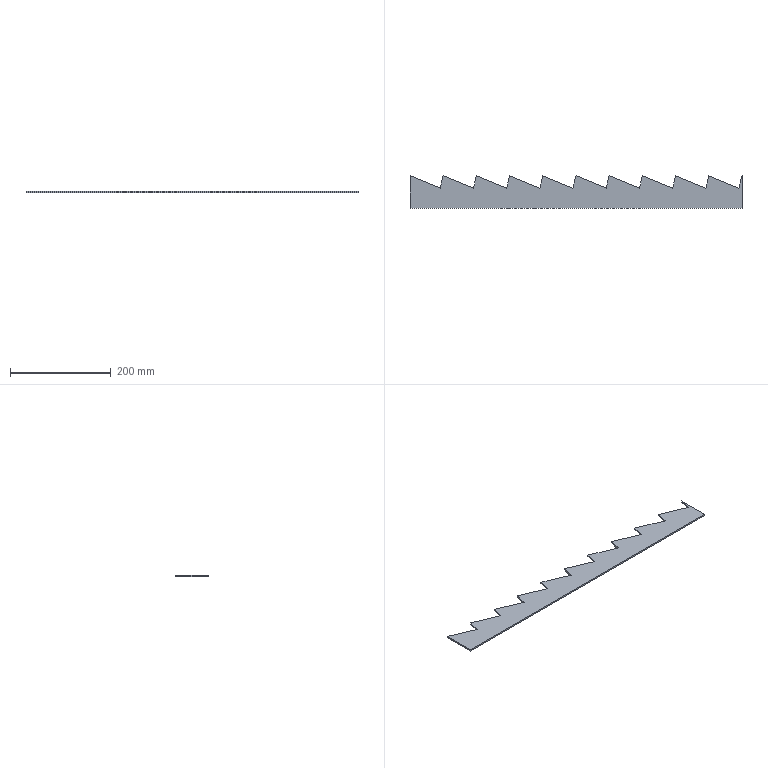Part | SolidWorks | features BaseBody 1 | 1 solid | 25 faces | box 660 x 65 x 3 mm | volume 103950 mm3 | plane 25
STEP:
#1=CARTESIAN_POINT('',(660.,-65.,0.));
#2=VERTEX_POINT('',#1);
#3=CARTESIAN_POINT('',(660.,0.,0.));
#4=VERTEX_POINT('',#3);
#5=CARTESIAN_POINT('',(660.,-32.5,0.));
#6=DIRECTION('',(0.,1.,0.));
#7=VECTOR('',#6,1000.);
#8=LINE('',#5,#7);
#9=EDGE_CURVE('',#2,#4,#8,.T.);
#10=ORIENTED_EDGE('',*,*,#9,.F.);
#11=CARTESIAN_POINT('',(0.,-65.,0.));
#12=VERTEX_POINT('',#11);
#13=CARTESIAN_POINT('',(330.,-65.,0.));
#14=DIRECTION('',(1.,0.,0.));
#15=VECTOR('',#14,1000.);
#16=LINE('',#13,#15);
#17=EDGE_CURVE('',#12,#2,#16,.T.);
#18=ORIENTED_EDGE('',*,*,#17,.F.);
#19=CARTESIAN_POINT('',(0.,0.,0.));
#20=VERTEX_POINT('',#19);
#21=CARTESIAN_POINT('',(0.,-32.5,0.));
#22=DIRECTION('',(0.,-1.,0.));
#23=VECTOR('',#22,1000.);
#24=LINE('',#21,#23);
#25=EDGE_CURVE('',#20,#12,#24,.T.);
#26=ORIENTED_EDGE('',*,*,#25,.F.);
#27=CARTESIAN_POINT('',(60.,-25.,0.));
#28=VERTEX_POINT('',#27);
#29=CARTESIAN_POINT('',(60.,-25.,0.));
#30=DIRECTION('',(-0.9231,0.3846,0.));
#31=VECTOR('',#30,1000.);
#32=LINE('',#29,#31);
#33=EDGE_CURVE('',#28,#20,#32,.T.);
#34=ORIENTED_EDGE('',*,*,#33,.F.);
#35=CARTESIAN_POINT('',(66.,0.,0.));
#36=VERTEX_POINT('',#35);
#37=CARTESIAN_POINT('',(66.,0.,0.));
#38=DIRECTION('',(-0.2334,-0.9724,0.));
#39=VECTOR('',#38,1000.);
#40=LINE('',#37,#39);
#41=EDGE_CURVE('',#36,#28,#40,.T.);
#42=ORIENTED_EDGE('',*,*,#41,.F.);
#43=CARTESIAN_POINT('',(126.,-25.,0.));
#44=VERTEX_POINT('',#43);
#45=CARTESIAN_POINT('',(126.,-25.,0.));
#46=DIRECTION('',(-0.9231,0.3846,0.));
#47=VECTOR('',#46,1000.);
#48=LINE('',#45,#47);
#49=EDGE_CURVE('',#44,#36,#48,.T.);
#50=ORIENTED_EDGE('',*,*,#49,.F.);
#51=CARTESIAN_POINT('',(132.,0.,0.));
#52=VERTEX_POINT('',#51);
#53=CARTESIAN_POINT('',(132.,0.,0.));
#54=DIRECTION('',(-0.2334,-0.9724,0.));
#55=VECTOR('',#54,1000.);
#56=LINE('',#53,#55);
#57=EDGE_CURVE('',#52,#44,#56,.T.);
#58=ORIENTED_EDGE('',*,*,#57,.F.);
#59=CARTESIAN_POINT('',(192.,-25.,0.));
#60=VERTEX_POINT('',#59);
#61=CARTESIAN_POINT('',(192.,-25.,0.));
#62=DIRECTION('',(-0.9231,0.3846,0.));
#63=VECTOR('',#62,1000.);
#64=LINE('',#61,#63);
#65=EDGE_CURVE('',#60,#52,#64,.T.);
#66=ORIENTED_EDGE('',*,*,#65,.F.);
#67=CARTESIAN_POINT('',(198.,0.,0.));
#68=VERTEX_POINT('',#67);
#69=CARTESIAN_POINT('',(198.,0.,0.));
#70=DIRECTION('',(-0.2334,-0.9724,0.));
#71=VECTOR('',#70,1000.);
#72=LINE('',#69,#71);
#73=EDGE_CURVE('',#68,#60,#72,.T.);
#74=ORIENTED_EDGE('',*,*,#73,.F.);
#75=CARTESIAN_POINT('',(258.,-25.,0.));
#76=VERTEX_POINT('',#75);
#77=CARTESIAN_POINT('',(258.,-25.,0.));
#78=DIRECTION('',(-0.9231,0.3846,0.));
#79=VECTOR('',#78,1000.);
#80=LINE('',#77,#79);
#81=EDGE_CURVE('',#76,#68,#80,.T.);
#82=ORIENTED_EDGE('',*,*,#81,.F.);
#83=CARTESIAN_POINT('',(264.,0.,0.));
#84=VERTEX_POINT('',#83);
#85=CARTESIAN_POINT('',(264.,0.,0.));
#86=DIRECTION('',(-0.2334,-0.9724,0.));
#87=VECTOR('',#86,1000.);
#88=LINE('',#85,#87);
#89=EDGE_CURVE('',#84,#76,#88,.T.);
#90=ORIENTED_EDGE('',*,*,#89,.F.);
#91=CARTESIAN_POINT('',(324.,-25.,0.));
#92=VERTEX_POINT('',#91);
#93=CARTESIAN_POINT('',(324.,-25.,0.));
#94=DIRECTION('',(-0.9231,0.3846,0.));
#95=VECTOR('',#94,1000.);
#96=LINE('',#93,#95);
#97=EDGE_CURVE('',#92,#84,#96,.T.);
#98=ORIENTED_EDGE('',*,*,#97,.F.);
#99=CARTESIAN_POINT('',(330.,0.,0.));
#100=VERTEX_POINT('',#99);
#101=CARTESIAN_POINT('',(330.,0.,0.));
#102=DIRECTION('',(-0.2334,-0.9724,0.));
#103=VECTOR('',#102,1000.);
#104=LINE('',#101,#103);
#105=EDGE_CURVE('',#100,#92,#104,.T.);
#106=ORIENTED_EDGE('',*,*,#105,.F.);
#107=CARTESIAN_POINT('',(390.,-25.,0.));
#108=VERTEX_POINT('',#107);
#109=CARTESIAN_POINT('',(390.,-25.,0.));
#110=DIRECTION('',(-0.9231,0.3846,0.));
#111=VECTOR('',#110,1000.);
#112=LINE('',#109,#111);
#113=EDGE_CURVE('',#108,#100,#112,.T.);
#114=ORIENTED_EDGE('',*,*,#113,.F.);
#115=CARTESIAN_POINT('',(396.,0.,0.));
#116=VERTEX_POINT('',#115);
#117=CARTESIAN_POINT('',(396.,0.,0.));
#118=DIRECTION('',(-0.2334,-0.9724,0.));
#119=VECTOR('',#118,1000.);
#120=LINE('',#117,#119);
#121=EDGE_CURVE('',#116,#108,#120,.T.);
#122=ORIENTED_EDGE('',*,*,#121,.F.);
#123=CARTESIAN_POINT('',(456.,-25.,0.));
#124=VERTEX_POINT('',#123);
#125=CARTESIAN_POINT('',(456.,-25.,0.));
#126=DIRECTION('',(-0.9231,0.3846,0.));
#127=VECTOR('',#126,1000.);
#128=LINE('',#125,#127);
#129=EDGE_CURVE('',#124,#116,#128,.T.);
#130=ORIENTED_EDGE('',*,*,#129,.F.);
#131=CARTESIAN_POINT('',(462.,0.,0.));
#132=VERTEX_POINT('',#131);
#133=CARTESIAN_POINT('',(462.,0.,0.));
#134=DIRECTION('',(-0.2334,-0.9724,0.));
#135=VECTOR('',#134,1000.);
#136=LINE('',#133,#135);
#137=EDGE_CURVE('',#132,#124,#136,.T.);
#138=ORIENTED_EDGE('',*,*,#137,.F.);
#139=CARTESIAN_POINT('',(522.,-25.,0.));
#140=VERTEX_POINT('',#139);
#141=CARTESIAN_POINT('',(522.,-25.,0.));
#142=DIRECTION('',(-0.9231,0.3846,0.));
#143=VECTOR('',#142,1000.);
#144=LINE('',#141,#143);
#145=EDGE_CURVE('',#140,#132,#144,.T.);
#146=ORIENTED_EDGE('',*,*,#145,.F.);
#147=CARTESIAN_POINT('',(528.,0.,0.));
#148=VERTEX_POINT('',#147);
#149=CARTESIAN_POINT('',(528.,0.,0.));
#150=DIRECTION('',(-0.2334,-0.9724,0.));
#151=VECTOR('',#150,1000.);
#152=LINE('',#149,#151);
#153=EDGE_CURVE('',#148,#140,#152,.T.);
#154=ORIENTED_EDGE('',*,*,#153,.F.);
#155=CARTESIAN_POINT('',(588.,-25.,0.));
#156=VERTEX_POINT('',#155);
#157=CARTESIAN_POINT('',(588.,-25.,0.));
#158=DIRECTION('',(-0.9231,0.3846,0.));
#159=VECTOR('',#158,1000.);
#160=LINE('',#157,#159);
#161=EDGE_CURVE('',#156,#148,#160,.T.);
#162=ORIENTED_EDGE('',*,*,#161,.F.);
#163=CARTESIAN_POINT('',(594.,0.,0.));
#164=VERTEX_POINT('',#163);
#165=CARTESIAN_POINT('',(594.,0.,0.));
#166=DIRECTION('',(-0.2334,-0.9724,0.));
#167=VECTOR('',#166,1000.);
#168=LINE('',#165,#167);
#169=EDGE_CURVE('',#164,#156,#168,.T.);
#170=ORIENTED_EDGE('',*,*,#169,.F.);
#171=CARTESIAN_POINT('',(654.,-25.,0.));
#172=VERTEX_POINT('',#171);
#173=CARTESIAN_POINT('',(654.,-25.,0.));
#174=DIRECTION('',(-0.9231,0.3846,0.));
#175=VECTOR('',#174,1000.);
#176=LINE('',#173,#175);
#177=EDGE_CURVE('',#172,#164,#176,.T.);
#178=ORIENTED_EDGE('',*,*,#177,.F.);
#179=CARTESIAN_POINT('',(660.,0.,0.));
#180=DIRECTION('',(-0.2334,-0.9724,0.));
#181=VECTOR('',#180,1000.);
#182=LINE('',#179,#181);
#183=EDGE_CURVE('',#4,#172,#182,.T.);
#184=ORIENTED_EDGE('',*,*,#183,.F.);
#185=EDGE_LOOP('',(#10,#18,#26,#34,#42,#50,#58,#66,#74,#82,#90,#98,#106,#114,#122,#130,#138,#146,#154,#162,#170,#178,#184));
#186=FACE_OUTER_BOUND('',#185,.T.);
#187=CARTESIAN_POINT('',(330.,-32.5,0.));
#188=DIRECTION('',(0.,0.,1.));
#189=DIRECTION('',(1.,0.,0.));
#190=AXIS2_PLACEMENT_3D('',#187,#188,#189);
#191=PLANE('',#190);
#192=ADVANCED_FACE('',(#186),#191,.F.);
#193=CARTESIAN_POINT('',(654.,-25.,3.));
#194=VERTEX_POINT('',#193);
#195=CARTESIAN_POINT('',(654.,-25.,3.));
#196=DIRECTION('',(0.,0.,-1.));
#197=VECTOR('',#196,1000.);
#198=LINE('',#195,#197);
#199=EDGE_CURVE('',#194,#172,#198,.T.);
#200=ORIENTED_EDGE('',*,*,#199,.F.);
#201=CARTESIAN_POINT('',(660.,0.,3.));
#202=VERTEX_POINT('',#201);
#203=CARTESIAN_POINT('',(660.,0.,3.));
#204=DIRECTION('',(-0.2334,-0.9724,0.));
#205=VECTOR('',#204,1000.);
#206=LINE('',#203,#205);
#207=EDGE_CURVE('',#202,#194,#206,.T.);
#208=ORIENTED_EDGE('',*,*,#207,.F.);
#209=CARTESIAN_POINT('',(660.,0.,3.));
#210=DIRECTION('',(0.,0.,1.));
#211=VECTOR('',#210,1000.);
#212=LINE('',#209,#211);
#213=EDGE_CURVE('',#4,#202,#212,.T.);
#214=ORIENTED_EDGE('',*,*,#213,.F.);
#215=ORIENTED_EDGE('',*,*,#183,.T.);
#216=EDGE_LOOP('',(#200,#208,#214,#215));
#217=FACE_OUTER_BOUND('',#216,.T.);
#218=CARTESIAN_POINT('',(660.,0.,3.));
#219=DIRECTION('',(0.9724,-0.2334,0.));
#220=DIRECTION('',(0.2334,0.9724,0.));
#221=AXIS2_PLACEMENT_3D('',#218,#219,#220);
#222=PLANE('',#221);
#223=ADVANCED_FACE('',(#217),#222,.F.);
#224=CARTESIAN_POINT('',(660.,-65.,3.));
#225=VERTEX_POINT('',#224);
#226=CARTESIAN_POINT('',(660.,-65.,3.));
#227=DIRECTION('',(0.,-1.,0.));
#228=VECTOR('',#227,1000.);
#229=LINE('',#226,#228);
#230=EDGE_CURVE('',#202,#225,#229,.T.);
#231=ORIENTED_EDGE('',*,*,#230,.T.);
#232=CARTESIAN_POINT('',(660.,-65.,0.));
#233=DIRECTION('',(0.,0.,-1.));
#234=VECTOR('',#233,1000.);
#235=LINE('',#232,#234);
#236=EDGE_CURVE('',#225,#2,#235,.T.);
#237=ORIENTED_EDGE('',*,*,#236,.T.);
#238=ORIENTED_EDGE('',*,*,#9,.T.);
#239=ORIENTED_EDGE('',*,*,#213,.T.);
#240=EDGE_LOOP('',(#231,#237,#238,#239));
#241=FACE_OUTER_BOUND('',#240,.T.);
#242=CARTESIAN_POINT('',(660.,-65.,0.));
#243=DIRECTION('',(1.,0.,0.));
#244=DIRECTION('',(0.,0.,-1.));
#245=AXIS2_PLACEMENT_3D('',#242,#243,#244);
#246=PLANE('',#245);
#247=ADVANCED_FACE('',(#241),#246,.T.);
#248=CARTESIAN_POINT('',(0.,-65.,3.));
#249=VERTEX_POINT('',#248);
#250=CARTESIAN_POINT('',(0.,-65.,3.));
#251=DIRECTION('',(-1.,0.,0.));
#252=VECTOR('',#251,1000.);
#253=LINE('',#250,#252);
#254=EDGE_CURVE('',#225,#249,#253,.T.);
#255=ORIENTED_EDGE('',*,*,#254,.T.);
#256=CARTESIAN_POINT('',(0.,-65.,0.));
#257=DIRECTION('',(0.,0.,-1.));
#258=VECTOR('',#257,1000.);
#259=LINE('',#256,#258);
#260=EDGE_CURVE('',#249,#12,#259,.T.);
#261=ORIENTED_EDGE('',*,*,#260,.T.);
#262=ORIENTED_EDGE('',*,*,#17,.T.);
#263=ORIENTED_EDGE('',*,*,#236,.F.);
#264=EDGE_LOOP('',(#255,#261,#262,#263));
#265=FACE_OUTER_BOUND('',#264,.T.);
#266=CARTESIAN_POINT('',(0.,-65.,0.));
#267=DIRECTION('',(0.,-1.,0.));
#268=DIRECTION('',(1.,0.,0.));
#269=AXIS2_PLACEMENT_3D('',#266,#267,#268);
#270=PLANE('',#269);
#271=ADVANCED_FACE('',(#265),#270,.T.);
#272=CARTESIAN_POINT('',(0.,0.,3.));
#273=VERTEX_POINT('',#272);
#274=CARTESIAN_POINT('',(0.,0.,3.));
#275=DIRECTION('',(0.,1.,0.));
#276=VECTOR('',#275,1000.);
#277=LINE('',#274,#276);
#278=EDGE_CURVE('',#249,#273,#277,.T.);
#279=ORIENTED_EDGE('',*,*,#278,.T.);
#280=CARTESIAN_POINT('',(0.,0.,0.));
#281=DIRECTION('',(0.,0.,-1.));
#282=VECTOR('',#281,1000.);
#283=LINE('',#280,#282);
#284=EDGE_CURVE('',#273,#20,#283,.T.);
#285=ORIENTED_EDGE('',*,*,#284,.T.);
#286=ORIENTED_EDGE('',*,*,#25,.T.);
#287=ORIENTED_EDGE('',*,*,#260,.F.);
#288=EDGE_LOOP('',(#279,#285,#286,#287));
#289=FACE_OUTER_BOUND('',#288,.T.);
#290=CARTESIAN_POINT('',(0.,0.,0.));
#291=DIRECTION('',(-1.,0.,0.));
#292=DIRECTION('',(0.,-1.,0.));
#293=AXIS2_PLACEMENT_3D('',#290,#291,#292);
#294=PLANE('',#293);
#295=ADVANCED_FACE('',(#289),#294,.T.);
#296=ORIENTED_EDGE('',*,*,#284,.F.);
#297=CARTESIAN_POINT('',(60.,-25.,3.));
#298=VERTEX_POINT('',#297);
#299=CARTESIAN_POINT('',(60.,-25.,3.));
#300=DIRECTION('',(-0.9231,0.3846,0.));
#301=VECTOR('',#300,1000.);
#302=LINE('',#299,#301);
#303=EDGE_CURVE('',#298,#273,#302,.T.);
#304=ORIENTED_EDGE('',*,*,#303,.F.);
#305=CARTESIAN_POINT('',(60.,-25.,3.));
#306=DIRECTION('',(0.,0.,1.));
#307=VECTOR('',#306,1000.);
#308=LINE('',#305,#307);
#309=EDGE_CURVE('',#28,#298,#308,.T.);
#310=ORIENTED_EDGE('',*,*,#309,.F.);
#311=ORIENTED_EDGE('',*,*,#33,.T.);
#312=EDGE_LOOP('',(#296,#304,#310,#311));
#313=FACE_OUTER_BOUND('',#312,.T.);
#314=CARTESIAN_POINT('',(60.,-25.,3.));
#315=DIRECTION('',(-0.3846,-0.9231,0.));
#316=DIRECTION('',(0.9231,-0.3846,0.));
#317=AXIS2_PLACEMENT_3D('',#314,#315,#316);
#318=PLANE('',#317);
#319=ADVANCED_FACE('',(#313),#318,.F.);
#320=ORIENTED_EDGE('',*,*,#309,.T.);
#321=CARTESIAN_POINT('',(66.,0.,3.));
#322=VERTEX_POINT('',#321);
#323=CARTESIAN_POINT('',(66.,0.,3.));
#324=DIRECTION('',(-0.2334,-0.9724,0.));
#325=VECTOR('',#324,1000.);
#326=LINE('',#323,#325);
#327=EDGE_CURVE('',#322,#298,#326,.T.);
#328=ORIENTED_EDGE('',*,*,#327,.F.);
#329=CARTESIAN_POINT('',(66.,0.,3.));
#330=DIRECTION('',(0.,0.,1.));
#331=VECTOR('',#330,1000.);
#332=LINE('',#329,#331);
#333=EDGE_CURVE('',#36,#322,#332,.T.);
#334=ORIENTED_EDGE('',*,*,#333,.F.);
#335=ORIENTED_EDGE('',*,*,#41,.T.);
#336=EDGE_LOOP('',(#320,#328,#334,#335));
#337=FACE_OUTER_BOUND('',#336,.T.);
#338=CARTESIAN_POINT('',(66.,0.,3.));
#339=DIRECTION('',(0.9724,-0.2334,0.));
#340=DIRECTION('',(0.2334,0.9724,0.));
#341=AXIS2_PLACEMENT_3D('',#338,#339,#340);
#342=PLANE('',#341);
#343=ADVANCED_FACE('',(#337),#342,.F.);
#344=ORIENTED_EDGE('',*,*,#333,.T.);
#345=CARTESIAN_POINT('',(126.,-25.,3.));
#346=VERTEX_POINT('',#345);
#347=CARTESIAN_POINT('',(126.,-25.,3.));
#348=DIRECTION('',(-0.9231,0.3846,0.));
#349=VECTOR('',#348,1000.);
#350=LINE('',#347,#349);
#351=EDGE_CURVE('',#346,#322,#350,.T.);
#352=ORIENTED_EDGE('',*,*,#351,.F.);
#353=CARTESIAN_POINT('',(126.,-25.,3.));
#354=DIRECTION('',(0.,0.,1.));
#355=VECTOR('',#354,1000.);
#356=LINE('',#353,#355);
#357=EDGE_CURVE('',#44,#346,#356,.T.);
#358=ORIENTED_EDGE('',*,*,#357,.F.);
#359=ORIENTED_EDGE('',*,*,#49,.T.);
#360=EDGE_LOOP('',(#344,#352,#358,#359));
#361=FACE_OUTER_BOUND('',#360,.T.);
#362=CARTESIAN_POINT('',(126.,-25.,3.));
#363=DIRECTION('',(-0.3846,-0.9231,0.));
#364=DIRECTION('',(0.9231,-0.3846,0.));
#365=AXIS2_PLACEMENT_3D('',#362,#363,#364);
#366=PLANE('',#365);
#367=ADVANCED_FACE('',(#361),#366,.F.);
#368=ORIENTED_EDGE('',*,*,#357,.T.);
#369=CARTESIAN_POINT('',(132.,0.,3.));
#370=VERTEX_POINT('',#369);
#371=CARTESIAN_POINT('',(132.,0.,3.));
#372=DIRECTION('',(-0.2334,-0.9724,0.));
#373=VECTOR('',#372,1000.);
#374=LINE('',#371,#373);
#375=EDGE_CURVE('',#370,#346,#374,.T.);
#376=ORIENTED_EDGE('',*,*,#375,.F.);
#377=CARTESIAN_POINT('',(132.,0.,3.));
#378=DIRECTION('',(0.,0.,1.));
#379=VECTOR('',#378,1000.);
#380=LINE('',#377,#379);
#381=EDGE_CURVE('',#52,#370,#380,.T.);
#382=ORIENTED_EDGE('',*,*,#381,.F.);
#383=ORIENTED_EDGE('',*,*,#57,.T.);
#384=EDGE_LOOP('',(#368,#376,#382,#383));
#385=FACE_OUTER_BOUND('',#384,.T.);
#386=CARTESIAN_POINT('',(132.,0.,3.));
#387=DIRECTION('',(0.9724,-0.2334,0.));
#388=DIRECTION('',(0.2334,0.9724,0.));
#389=AXIS2_PLACEMENT_3D('',#386,#387,#388);
#390=PLANE('',#389);
#391=ADVANCED_FACE('',(#385),#390,.F.);
#392=ORIENTED_EDGE('',*,*,#381,.T.);
#393=CARTESIAN_POINT('',(192.,-25.,3.));
#394=VERTEX_POINT('',#393);
#395=CARTESIAN_POINT('',(192.,-25.,3.));
#396=DIRECTION('',(-0.9231,0.3846,0.));
#397=VECTOR('',#396,1000.);
#398=LINE('',#395,#397);
#399=EDGE_CURVE('',#394,#370,#398,.T.);
#400=ORIENTED_EDGE('',*,*,#399,.F.);
#401=CARTESIAN_POINT('',(192.,-25.,3.));
#402=DIRECTION('',(0.,0.,1.));
#403=VECTOR('',#402,1000.);
#404=LINE('',#401,#403);
#405=EDGE_CURVE('',#60,#394,#404,.T.);
#406=ORIENTED_EDGE('',*,*,#405,.F.);
#407=ORIENTED_EDGE('',*,*,#65,.T.);
#408=EDGE_LOOP('',(#392,#400,#406,#407));
#409=FACE_OUTER_BOUND('',#408,.T.);
#410=CARTESIAN_POINT('',(192.,-25.,3.));
#411=DIRECTION('',(-0.3846,-0.9231,0.));
#412=DIRECTION('',(0.9231,-0.3846,0.));
#413=AXIS2_PLACEMENT_3D('',#410,#411,#412);
#414=PLANE('',#413);
#415=ADVANCED_FACE('',(#409),#414,.F.);
#416=ORIENTED_EDGE('',*,*,#405,.T.);
#417=CARTESIAN_POINT('',(198.,0.,3.));
#418=VERTEX_POINT('',#417);
#419=CARTESIAN_POINT('',(198.,0.,3.));
#420=DIRECTION('',(-0.2334,-0.9724,0.));
#421=VECTOR('',#420,1000.);
#422=LINE('',#419,#421);
#423=EDGE_CURVE('',#418,#394,#422,.T.);
#424=ORIENTED_EDGE('',*,*,#423,.F.);
#425=CARTESIAN_POINT('',(198.,0.,3.));
#426=DIRECTION('',(0.,0.,1.));
#427=VECTOR('',#426,1000.);
#428=LINE('',#425,#427);
#429=EDGE_CURVE('',#68,#418,#428,.T.);
#430=ORIENTED_EDGE('',*,*,#429,.F.);
#431=ORIENTED_EDGE('',*,*,#73,.T.);
#432=EDGE_LOOP('',(#416,#424,#430,#431));
#433=FACE_OUTER_BOUND('',#432,.T.);
#434=CARTESIAN_POINT('',(198.,0.,3.));
#435=DIRECTION('',(0.9724,-0.2334,0.));
#436=DIRECTION('',(0.2334,0.9724,0.));
#437=AXIS2_PLACEMENT_3D('',#434,#435,#436);
#438=PLANE('',#437);
#439=ADVANCED_FACE('',(#433),#438,.F.);
#440=ORIENTED_EDGE('',*,*,#429,.T.);
#441=CARTESIAN_POINT('',(258.,-25.,3.));
#442=VERTEX_POINT('',#441);
#443=CARTESIAN_POINT('',(258.,-25.,3.));
#444=DIRECTION('',(-0.9231,0.3846,0.));
#445=VECTOR('',#444,1000.);
#446=LINE('',#443,#445);
#447=EDGE_CURVE('',#442,#418,#446,.T.);
#448=ORIENTED_EDGE('',*,*,#447,.F.);
#449=CARTESIAN_POINT('',(258.,-25.,3.));
#450=DIRECTION('',(0.,0.,1.));
#451=VECTOR('',#450,1000.);
#452=LINE('',#449,#451);
#453=EDGE_CURVE('',#76,#442,#452,.T.);
#454=ORIENTED_EDGE('',*,*,#453,.F.);
#455=ORIENTED_EDGE('',*,*,#81,.T.);
#456=EDGE_LOOP('',(#440,#448,#454,#455));
#457=FACE_OUTER_BOUND('',#456,.T.);
#458=CARTESIAN_POINT('',(258.,-25.,3.));
#459=DIRECTION('',(-0.3846,-0.9231,0.));
#460=DIRECTION('',(0.9231,-0.3846,0.));
#461=AXIS2_PLACEMENT_3D('',#458,#459,#460);
#462=PLANE('',#461);
#463=ADVANCED_FACE('',(#457),#462,.F.);
#464=ORIENTED_EDGE('',*,*,#453,.T.);
#465=CARTESIAN_POINT('',(264.,0.,3.));
#466=VERTEX_POINT('',#465);
#467=CARTESIAN_POINT('',(264.,0.,3.));
#468=DIRECTION('',(-0.2334,-0.9724,0.));
#469=VECTOR('',#468,1000.);
#470=LINE('',#467,#469);
#471=EDGE_CURVE('',#466,#442,#470,.T.);
#472=ORIENTED_EDGE('',*,*,#471,.F.);
#473=CARTESIAN_POINT('',(264.,0.,3.));
#474=DIRECTION('',(0.,0.,1.));
#475=VECTOR('',#474,1000.);
#476=LINE('',#473,#475);
#477=EDGE_CURVE('',#84,#466,#476,.T.);
#478=ORIENTED_EDGE('',*,*,#477,.F.);
#479=ORIENTED_EDGE('',*,*,#89,.T.);
#480=EDGE_LOOP('',(#464,#472,#478,#479));
#481=FACE_OUTER_BOUND('',#480,.T.);
#482=CARTESIAN_POINT('',(264.,0.,3.));
#483=DIRECTION('',(0.9724,-0.2334,0.));
#484=DIRECTION('',(0.2334,0.9724,0.));
#485=AXIS2_PLACEMENT_3D('',#482,#483,#484);
#486=PLANE('',#485);
#487=ADVANCED_FACE('',(#481),#486,.F.);
#488=ORIENTED_EDGE('',*,*,#477,.T.);
#489=CARTESIAN_POINT('',(324.,-25.,3.));
#490=VERTEX_POINT('',#489);
#491=CARTESIAN_POINT('',(324.,-25.,3.));
#492=DIRECTION('',(-0.9231,0.3846,0.));
#493=VECTOR('',#492,1000.);
#494=LINE('',#491,#493);
#495=EDGE_CURVE('',#490,#466,#494,.T.);
#496=ORIENTED_EDGE('',*,*,#495,.F.);
#497=CARTESIAN_POINT('',(324.,-25.,3.));
#498=DIRECTION('',(0.,0.,1.));
#499=VECTOR('',#498,1000.);
#500=LINE('',#497,#499);
#501=EDGE_CURVE('',#92,#490,#500,.T.);
#502=ORIENTED_EDGE('',*,*,#501,.F.);
#503=ORIENTED_EDGE('',*,*,#97,.T.);
#504=EDGE_LOOP('',(#488,#496,#502,#503));
#505=FACE_OUTER_BOUND('',#504,.T.);
#506=CARTESIAN_POINT('',(324.,-25.,3.));
#507=DIRECTION('',(-0.3846,-0.9231,0.));
#508=DIRECTION('',(0.9231,-0.3846,0.));
#509=AXIS2_PLACEMENT_3D('',#506,#507,#508);
#510=PLANE('',#509);
#511=ADVANCED_FACE('',(#505),#510,.F.);
#512=ORIENTED_EDGE('',*,*,#501,.T.);
#513=CARTESIAN_POINT('',(330.,0.,3.));
#514=VERTEX_POINT('',#513);
#515=CARTESIAN_POINT('',(330.,0.,3.));
#516=DIRECTION('',(-0.2334,-0.9724,0.));
#517=VECTOR('',#516,1000.);
#518=LINE('',#515,#517);
#519=EDGE_CURVE('',#514,#490,#518,.T.);
#520=ORIENTED_EDGE('',*,*,#519,.F.);
#521=CARTESIAN_POINT('',(330.,0.,3.));
#522=DIRECTION('',(0.,0.,1.));
#523=VECTOR('',#522,1000.);
#524=LINE('',#521,#523);
#525=EDGE_CURVE('',#100,#514,#524,.T.);
#526=ORIENTED_EDGE('',*,*,#525,.F.);
#527=ORIENTED_EDGE('',*,*,#105,.T.);
#528=EDGE_LOOP('',(#512,#520,#526,#527));
#529=FACE_OUTER_BOUND('',#528,.T.);
#530=CARTESIAN_POINT('',(330.,0.,3.));
#531=DIRECTION('',(0.9724,-0.2334,0.));
#532=DIRECTION('',(0.2334,0.9724,0.));
#533=AXIS2_PLACEMENT_3D('',#530,#531,#532);
#534=PLANE('',#533);
#535=ADVANCED_FACE('',(#529),#534,.F.);
#536=ORIENTED_EDGE('',*,*,#525,.T.);
#537=CARTESIAN_POINT('',(390.,-25.,3.));
#538=VERTEX_POINT('',#537);
#539=CARTESIAN_POINT('',(390.,-25.,3.));
#540=DIRECTION('',(-0.9231,0.3846,0.));
#541=VECTOR('',#540,1000.);
#542=LINE('',#539,#541);
#543=EDGE_CURVE('',#538,#514,#542,.T.);
#544=ORIENTED_EDGE('',*,*,#543,.F.);
#545=CARTESIAN_POINT('',(390.,-25.,3.));
#546=DIRECTION('',(0.,0.,1.));
#547=VECTOR('',#546,1000.);
#548=LINE('',#545,#547);
#549=EDGE_CURVE('',#108,#538,#548,.T.);
#550=ORIENTED_EDGE('',*,*,#549,.F.);
#551=ORIENTED_EDGE('',*,*,#113,.T.);
#552=EDGE_LOOP('',(#536,#544,#550,#551));
#553=FACE_OUTER_BOUND('',#552,.T.);
#554=CARTESIAN_POINT('',(390.,-25.,3.));
#555=DIRECTION('',(-0.3846,-0.9231,0.));
#556=DIRECTION('',(0.9231,-0.3846,0.));
#557=AXIS2_PLACEMENT_3D('',#554,#555,#556);
#558=PLANE('',#557);
#559=ADVANCED_FACE('',(#553),#558,.F.);
#560=ORIENTED_EDGE('',*,*,#549,.T.);
#561=CARTESIAN_POINT('',(396.,0.,3.));
#562=VERTEX_POINT('',#561);
#563=CARTESIAN_POINT('',(396.,0.,3.));
#564=DIRECTION('',(-0.2334,-0.9724,0.));
#565=VECTOR('',#564,1000.);
#566=LINE('',#563,#565);
#567=EDGE_CURVE('',#562,#538,#566,.T.);
#568=ORIENTED_EDGE('',*,*,#567,.F.);
#569=CARTESIAN_POINT('',(396.,0.,3.));
#570=DIRECTION('',(0.,0.,1.));
#571=VECTOR('',#570,1000.);
#572=LINE('',#569,#571);
#573=EDGE_CURVE('',#116,#562,#572,.T.);
#574=ORIENTED_EDGE('',*,*,#573,.F.);
#575=ORIENTED_EDGE('',*,*,#121,.T.);
#576=EDGE_LOOP('',(#560,#568,#574,#575));
#577=FACE_OUTER_BOUND('',#576,.T.);
#578=CARTESIAN_POINT('',(396.,0.,3.));
#579=DIRECTION('',(0.9724,-0.2334,0.));
#580=DIRECTION('',(0.2334,0.9724,0.));
#581=AXIS2_PLACEMENT_3D('',#578,#579,#580);
#582=PLANE('',#581);
#583=ADVANCED_FACE('',(#577),#582,.F.);
#584=ORIENTED_EDGE('',*,*,#573,.T.);
#585=CARTESIAN_POINT('',(456.,-25.,3.));
#586=VERTEX_POINT('',#585);
#587=CARTESIAN_POINT('',(456.,-25.,3.));
#588=DIRECTION('',(-0.9231,0.3846,0.));
#589=VECTOR('',#588,1000.);
#590=LINE('',#587,#589);
#591=EDGE_CURVE('',#586,#562,#590,.T.);
#592=ORIENTED_EDGE('',*,*,#591,.F.);
#593=CARTESIAN_POINT('',(456.,-25.,3.));
#594=DIRECTION('',(0.,0.,1.));
#595=VECTOR('',#594,1000.);
#596=LINE('',#593,#595);
#597=EDGE_CURVE('',#124,#586,#596,.T.);
#598=ORIENTED_EDGE('',*,*,#597,.F.);
#599=ORIENTED_EDGE('',*,*,#129,.T.);
#600=EDGE_LOOP('',(#584,#592,#598,#599));
#601=FACE_OUTER_BOUND('',#600,.T.);
#602=CARTESIAN_POINT('',(456.,-25.,3.));
#603=DIRECTION('',(-0.3846,-0.9231,0.));
#604=DIRECTION('',(0.9231,-0.3846,0.));
#605=AXIS2_PLACEMENT_3D('',#602,#603,#604);
#606=PLANE('',#605);
#607=ADVANCED_FACE('',(#601),#606,.F.);
#608=ORIENTED_EDGE('',*,*,#597,.T.);
#609=CARTESIAN_POINT('',(462.,0.,3.));
#610=VERTEX_POINT('',#609);
#611=CARTESIAN_POINT('',(462.,0.,3.));
#612=DIRECTION('',(-0.2334,-0.9724,0.));
#613=VECTOR('',#612,1000.);
#614=LINE('',#611,#613);
#615=EDGE_CURVE('',#610,#586,#614,.T.);
#616=ORIENTED_EDGE('',*,*,#615,.F.);
#617=CARTESIAN_POINT('',(462.,0.,3.));
#618=DIRECTION('',(0.,0.,1.));
#619=VECTOR('',#618,1000.);
#620=LINE('',#617,#619);
#621=EDGE_CURVE('',#132,#610,#620,.T.);
#622=ORIENTED_EDGE('',*,*,#621,.F.);
#623=ORIENTED_EDGE('',*,*,#137,.T.);
#624=EDGE_LOOP('',(#608,#616,#622,#623));
#625=FACE_OUTER_BOUND('',#624,.T.);
#626=CARTESIAN_POINT('',(462.,0.,3.));
#627=DIRECTION('',(0.9724,-0.2334,0.));
#628=DIRECTION('',(0.2334,0.9724,0.));
#629=AXIS2_PLACEMENT_3D('',#626,#627,#628);
#630=PLANE('',#629);
#631=ADVANCED_FACE('',(#625),#630,.F.);
#632=ORIENTED_EDGE('',*,*,#621,.T.);
#633=CARTESIAN_POINT('',(522.,-25.,3.));
#634=VERTEX_POINT('',#633);
#635=CARTESIAN_POINT('',(522.,-25.,3.));
#636=DIRECTION('',(-0.9231,0.3846,0.));
#637=VECTOR('',#636,1000.);
#638=LINE('',#635,#637);
#639=EDGE_CURVE('',#634,#610,#638,.T.);
#640=ORIENTED_EDGE('',*,*,#639,.F.);
#641=CARTESIAN_POINT('',(522.,-25.,3.));
#642=DIRECTION('',(0.,0.,1.));
#643=VECTOR('',#642,1000.);
#644=LINE('',#641,#643);
#645=EDGE_CURVE('',#140,#634,#644,.T.);
#646=ORIENTED_EDGE('',*,*,#645,.F.);
#647=ORIENTED_EDGE('',*,*,#145,.T.);
#648=EDGE_LOOP('',(#632,#640,#646,#647));
#649=FACE_OUTER_BOUND('',#648,.T.);
#650=CARTESIAN_POINT('',(522.,-25.,3.));
#651=DIRECTION('',(-0.3846,-0.9231,0.));
#652=DIRECTION('',(0.9231,-0.3846,0.));
#653=AXIS2_PLACEMENT_3D('',#650,#651,#652);
#654=PLANE('',#653);
#655=ADVANCED_FACE('',(#649),#654,.F.);
#656=ORIENTED_EDGE('',*,*,#645,.T.);
#657=CARTESIAN_POINT('',(528.,0.,3.));
#658=VERTEX_POINT('',#657);
#659=CARTESIAN_POINT('',(528.,0.,3.));
#660=DIRECTION('',(-0.2334,-0.9724,0.));
#661=VECTOR('',#660,1000.);
#662=LINE('',#659,#661);
#663=EDGE_CURVE('',#658,#634,#662,.T.);
#664=ORIENTED_EDGE('',*,*,#663,.F.);
#665=CARTESIAN_POINT('',(528.,0.,3.));
#666=DIRECTION('',(0.,0.,1.));
#667=VECTOR('',#666,1000.);
#668=LINE('',#665,#667);
#669=EDGE_CURVE('',#148,#658,#668,.T.);
#670=ORIENTED_EDGE('',*,*,#669,.F.);
#671=ORIENTED_EDGE('',*,*,#153,.T.);
#672=EDGE_LOOP('',(#656,#664,#670,#671));
#673=FACE_OUTER_BOUND('',#672,.T.);
#674=CARTESIAN_POINT('',(528.,0.,3.));
#675=DIRECTION('',(0.9724,-0.2334,0.));
#676=DIRECTION('',(0.2334,0.9724,0.));
#677=AXIS2_PLACEMENT_3D('',#674,#675,#676);
#678=PLANE('',#677);
#679=ADVANCED_FACE('',(#673),#678,.F.);
#680=ORIENTED_EDGE('',*,*,#669,.T.);
#681=CARTESIAN_POINT('',(588.,-25.,3.));
#682=VERTEX_POINT('',#681);
#683=CARTESIAN_POINT('',(588.,-25.,3.));
#684=DIRECTION('',(-0.9231,0.3846,0.));
#685=VECTOR('',#684,1000.);
#686=LINE('',#683,#685);
#687=EDGE_CURVE('',#682,#658,#686,.T.);
#688=ORIENTED_EDGE('',*,*,#687,.F.);
#689=CARTESIAN_POINT('',(588.,-25.,3.));
#690=DIRECTION('',(0.,0.,1.));
#691=VECTOR('',#690,1000.);
#692=LINE('',#689,#691);
#693=EDGE_CURVE('',#156,#682,#692,.T.);
#694=ORIENTED_EDGE('',*,*,#693,.F.);
#695=ORIENTED_EDGE('',*,*,#161,.T.);
#696=EDGE_LOOP('',(#680,#688,#694,#695));
#697=FACE_OUTER_BOUND('',#696,.T.);
#698=CARTESIAN_POINT('',(588.,-25.,3.));
#699=DIRECTION('',(-0.3846,-0.9231,0.));
#700=DIRECTION('',(0.9231,-0.3846,0.));
#701=AXIS2_PLACEMENT_3D('',#698,#699,#700);
#702=PLANE('',#701);
#703=ADVANCED_FACE('',(#697),#702,.F.);
#704=ORIENTED_EDGE('',*,*,#693,.T.);
#705=CARTESIAN_POINT('',(594.,0.,3.));
#706=VERTEX_POINT('',#705);
#707=CARTESIAN_POINT('',(594.,0.,3.));
#708=DIRECTION('',(-0.2334,-0.9724,0.));
#709=VECTOR('',#708,1000.);
#710=LINE('',#707,#709);
#711=EDGE_CURVE('',#706,#682,#710,.T.);
#712=ORIENTED_EDGE('',*,*,#711,.F.);
#713=CARTESIAN_POINT('',(594.,0.,3.));
#714=DIRECTION('',(0.,0.,1.));
#715=VECTOR('',#714,1000.);
#716=LINE('',#713,#715);
#717=EDGE_CURVE('',#164,#706,#716,.T.);
#718=ORIENTED_EDGE('',*,*,#717,.F.);
#719=ORIENTED_EDGE('',*,*,#169,.T.);
#720=EDGE_LOOP('',(#704,#712,#718,#719));
#721=FACE_OUTER_BOUND('',#720,.T.);
#722=CARTESIAN_POINT('',(594.,0.,3.));
#723=DIRECTION('',(0.9724,-0.2334,0.));
#724=DIRECTION('',(0.2334,0.9724,0.));
#725=AXIS2_PLACEMENT_3D('',#722,#723,#724);
#726=PLANE('',#725);
#727=ADVANCED_FACE('',(#721),#726,.F.);
#728=ORIENTED_EDGE('',*,*,#717,.T.);
#729=CARTESIAN_POINT('',(654.,-25.,3.));
#730=DIRECTION('',(-0.9231,0.3846,0.));
#731=VECTOR('',#730,1000.);
#732=LINE('',#729,#731);
#733=EDGE_CURVE('',#194,#706,#732,.T.);
#734=ORIENTED_EDGE('',*,*,#733,.F.);
#735=ORIENTED_EDGE('',*,*,#199,.T.);
#736=ORIENTED_EDGE('',*,*,#177,.T.);
#737=EDGE_LOOP('',(#728,#734,#735,#736));
#738=FACE_OUTER_BOUND('',#737,.T.);
#739=CARTESIAN_POINT('',(654.,-25.,3.));
#740=DIRECTION('',(-0.3846,-0.9231,0.));
#741=DIRECTION('',(0.9231,-0.3846,0.));
#742=AXIS2_PLACEMENT_3D('',#739,#740,#741);
#743=PLANE('',#742);
#744=ADVANCED_FACE('',(#738),#743,.F.);
#745=ORIENTED_EDGE('',*,*,#254,.F.);
#746=ORIENTED_EDGE('',*,*,#230,.F.);
#747=ORIENTED_EDGE('',*,*,#207,.T.);
#748=ORIENTED_EDGE('',*,*,#733,.T.);
#749=ORIENTED_EDGE('',*,*,#711,.T.);
#750=ORIENTED_EDGE('',*,*,#687,.T.);
#751=ORIENTED_EDGE('',*,*,#663,.T.);
#752=ORIENTED_EDGE('',*,*,#639,.T.);
#753=ORIENTED_EDGE('',*,*,#615,.T.);
#754=ORIENTED_EDGE('',*,*,#591,.T.);
#755=ORIENTED_EDGE('',*,*,#567,.T.);
#756=ORIENTED_EDGE('',*,*,#543,.T.);
#757=ORIENTED_EDGE('',*,*,#519,.T.);
#758=ORIENTED_EDGE('',*,*,#495,.T.);
#759=ORIENTED_EDGE('',*,*,#471,.T.);
#760=ORIENTED_EDGE('',*,*,#447,.T.);
#761=ORIENTED_EDGE('',*,*,#423,.T.);
#762=ORIENTED_EDGE('',*,*,#399,.T.);
#763=ORIENTED_EDGE('',*,*,#375,.T.);
#764=ORIENTED_EDGE('',*,*,#351,.T.);
#765=ORIENTED_EDGE('',*,*,#327,.T.);
#766=ORIENTED_EDGE('',*,*,#303,.T.);
#767=ORIENTED_EDGE('',*,*,#278,.F.);
#768=EDGE_LOOP('',(#745,#746,#747,#748,#749,#750,#751,#752,#753,#754,#755,#756,#757,#758,#759,#760,#761,#762,#763,#764,#765,#766,#767));
#769=FACE_OUTER_BOUND('',#768,.T.);
#770=CARTESIAN_POINT('',(330.,-32.5,3.));
#771=DIRECTION('',(0.,0.,1.));
#772=DIRECTION('',(1.,0.,0.));
#773=AXIS2_PLACEMENT_3D('',#770,#771,#772);
#774=PLANE('',#773);
#775=ADVANCED_FACE('',(#769),#774,.T.);
#776=CLOSED_SHELL('',(#192,#223,#247,#271,#295,#319,#343,#367,#391,#415,#439,#463,#487,#511,#535,#559,#583,#607,#631,#655,#679,#703,#727,#744,#775));
#777=MANIFOLD_SOLID_BREP('',#776);
#778=CARTESIAN_POINT('',(0.,0.,0.));
#779=DIRECTION('',(0.,0.,1.));
#780=DIRECTION('',(1.,0.,0.));
#781=AXIS2_PLACEMENT_3D('',#778,#779,#780);
#782=(LENGTH_UNIT()NAMED_UNIT(*)SI_UNIT(.MILLI.,.METRE.));
#783=UNCERTAINTY_MEASURE_WITH_UNIT(LENGTH_MEASURE(0.00001),#782,'','');
#784=(NAMED_UNIT(*)PLANE_ANGLE_UNIT()SI_UNIT($,.RADIAN.));
#785=(NAMED_UNIT(*)SI_UNIT($,.STERADIAN.)SOLID_ANGLE_UNIT());
#786=(GEOMETRIC_REPRESENTATION_CONTEXT(3)GLOBAL_UNCERTAINTY_ASSIGNED_CONTEXT((#783))GLOBAL_UNIT_ASSIGNED_CONTEXT((#782,#784,#785))REPRESENTATION_CONTEXT('',''));
#787=ADVANCED_BREP_SHAPE_REPRESENTATION('',(#777,#781),#786);